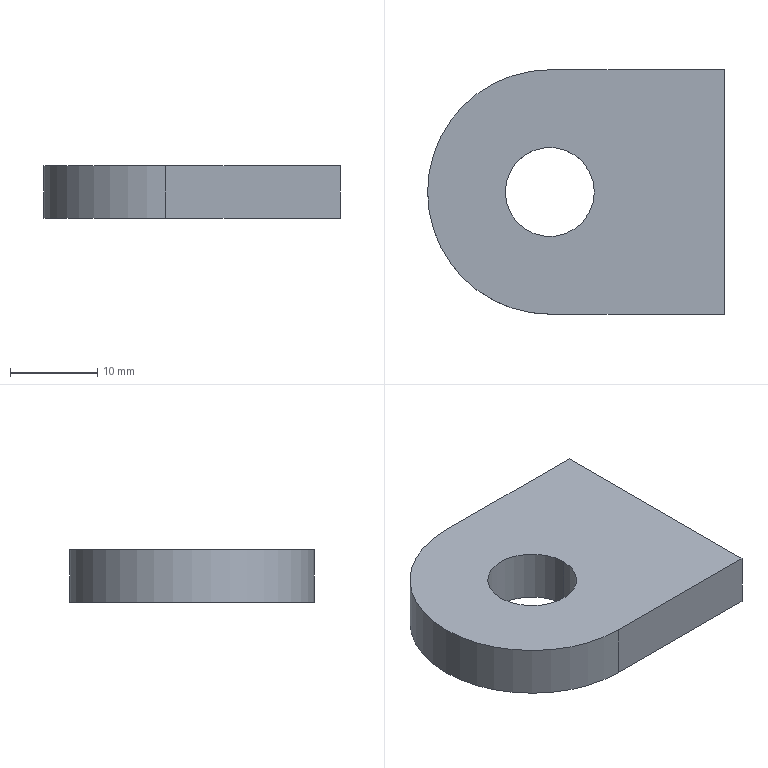Part | SolidWorks | features Extrusion 1 | 1 solid | 8 faces | box 34 x 28 x 6 mm | volume 4717 mm3 | plane 5 | cylinder 3 | commonest cylinder face diameters 10.2 x2 28 x1
STEP:
#1=CARTESIAN_POINT('',(-5.1,0.,-3.));
#2=VERTEX_POINT('',#1);
#3=CARTESIAN_POINT('',(5.1,0.,-3.));
#4=VERTEX_POINT('',#3);
#5=CARTESIAN_POINT('',(0.,0.,-3.));
#6=DIRECTION('',(0.,0.,1.));
#7=DIRECTION('',(1.,0.,0.));
#8=AXIS2_PLACEMENT_3D('',#5,#6,#7);
#9=CIRCLE('',#8,5.1);
#10=EDGE_CURVE('',#2,#4,#9,.T.);
#11=ORIENTED_EDGE('',*,*,#10,.F.);
#12=CARTESIAN_POINT('',(-5.1,0.,3.));
#13=VERTEX_POINT('',#12);
#14=CARTESIAN_POINT('',(-5.1,0.,-3.));
#15=DIRECTION('',(0.,0.,1.));
#16=VECTOR('',#15,1000.);
#17=LINE('',#14,#16);
#18=EDGE_CURVE('',#2,#13,#17,.T.);
#19=ORIENTED_EDGE('',*,*,#18,.T.);
#20=CARTESIAN_POINT('',(5.1,0.,3.));
#21=VERTEX_POINT('',#20);
#22=CARTESIAN_POINT('',(0.,0.,3.));
#23=DIRECTION('',(0.,0.,1.));
#24=DIRECTION('',(1.,0.,0.));
#25=AXIS2_PLACEMENT_3D('',#22,#23,#24);
#26=CIRCLE('',#25,5.1);
#27=EDGE_CURVE('',#13,#21,#26,.T.);
#28=ORIENTED_EDGE('',*,*,#27,.T.);
#29=CARTESIAN_POINT('',(5.1,0.,-3.));
#30=DIRECTION('',(0.,0.,1.));
#31=VECTOR('',#30,1000.);
#32=LINE('',#29,#31);
#33=EDGE_CURVE('',#4,#21,#32,.T.);
#34=ORIENTED_EDGE('',*,*,#33,.F.);
#35=EDGE_LOOP('',(#11,#19,#28,#34));
#36=FACE_OUTER_BOUND('',#35,.T.);
#37=CARTESIAN_POINT('',(0.,0.,-3.));
#38=DIRECTION('',(0.,0.,1.));
#39=DIRECTION('',(1.,0.,0.));
#40=AXIS2_PLACEMENT_3D('',#37,#38,#39);
#41=CYLINDRICAL_SURFACE('',#40,5.1);
#42=ADVANCED_FACE('',(#36),#41,.F.);
#43=CARTESIAN_POINT('',(0.,14.,3.));
#44=VERTEX_POINT('',#43);
#45=CARTESIAN_POINT('',(0.,-14.,3.));
#46=VERTEX_POINT('',#45);
#47=CARTESIAN_POINT('',(0.,0.,3.));
#48=DIRECTION('',(0.,0.,1.));
#49=DIRECTION('',(-1.,0.,0.));
#50=AXIS2_PLACEMENT_3D('',#47,#48,#49);
#51=CIRCLE('',#50,14.);
#52=EDGE_CURVE('',#44,#46,#51,.T.);
#53=ORIENTED_EDGE('',*,*,#52,.F.);
#54=CARTESIAN_POINT('',(0.,14.,-3.));
#55=VERTEX_POINT('',#54);
#56=CARTESIAN_POINT('',(0.,14.,-3.));
#57=DIRECTION('',(0.,0.,1.));
#58=VECTOR('',#57,1000.);
#59=LINE('',#56,#58);
#60=EDGE_CURVE('',#55,#44,#59,.T.);
#61=ORIENTED_EDGE('',*,*,#60,.F.);
#62=CARTESIAN_POINT('',(0.,-14.,-3.));
#63=VERTEX_POINT('',#62);
#64=CARTESIAN_POINT('',(0.,0.,-3.));
#65=DIRECTION('',(0.,0.,1.));
#66=DIRECTION('',(-1.,0.,0.));
#67=AXIS2_PLACEMENT_3D('',#64,#65,#66);
#68=CIRCLE('',#67,14.);
#69=EDGE_CURVE('',#55,#63,#68,.T.);
#70=ORIENTED_EDGE('',*,*,#69,.T.);
#71=CARTESIAN_POINT('',(0.,-14.,-3.));
#72=DIRECTION('',(0.,0.,1.));
#73=VECTOR('',#72,1000.);
#74=LINE('',#71,#73);
#75=EDGE_CURVE('',#63,#46,#74,.T.);
#76=ORIENTED_EDGE('',*,*,#75,.T.);
#77=EDGE_LOOP('',(#53,#61,#70,#76));
#78=FACE_OUTER_BOUND('',#77,.T.);
#79=CARTESIAN_POINT('',(0.,0.,-3.));
#80=DIRECTION('',(0.,0.,1.));
#81=DIRECTION('',(1.,0.,0.));
#82=AXIS2_PLACEMENT_3D('',#79,#80,#81);
#83=CYLINDRICAL_SURFACE('',#82,14.);
#84=ADVANCED_FACE('',(#78),#83,.T.);
#85=CARTESIAN_POINT('',(20.,14.,3.));
#86=VERTEX_POINT('',#85);
#87=CARTESIAN_POINT('',(0.,14.,3.));
#88=DIRECTION('',(-1.,0.,0.));
#89=VECTOR('',#88,1000.);
#90=LINE('',#87,#89);
#91=EDGE_CURVE('',#86,#44,#90,.T.);
#92=ORIENTED_EDGE('',*,*,#91,.F.);
#93=CARTESIAN_POINT('',(20.,14.,-3.));
#94=VERTEX_POINT('',#93);
#95=CARTESIAN_POINT('',(20.,14.,-3.));
#96=DIRECTION('',(0.,0.,1.));
#97=VECTOR('',#96,1000.);
#98=LINE('',#95,#97);
#99=EDGE_CURVE('',#94,#86,#98,.T.);
#100=ORIENTED_EDGE('',*,*,#99,.F.);
#101=CARTESIAN_POINT('',(0.,14.,-3.));
#102=DIRECTION('',(-1.,0.,0.));
#103=VECTOR('',#102,1000.);
#104=LINE('',#101,#103);
#105=EDGE_CURVE('',#94,#55,#104,.T.);
#106=ORIENTED_EDGE('',*,*,#105,.T.);
#107=ORIENTED_EDGE('',*,*,#60,.T.);
#108=EDGE_LOOP('',(#92,#100,#106,#107));
#109=FACE_OUTER_BOUND('',#108,.T.);
#110=CARTESIAN_POINT('',(0.,14.,-3.));
#111=DIRECTION('',(0.,1.,0.));
#112=DIRECTION('',(0.,0.,1.));
#113=AXIS2_PLACEMENT_3D('',#110,#111,#112);
#114=PLANE('',#113);
#115=ADVANCED_FACE('',(#109),#114,.T.);
#116=CARTESIAN_POINT('',(20.,-14.,3.));
#117=VERTEX_POINT('',#116);
#118=CARTESIAN_POINT('',(20.,14.,3.));
#119=DIRECTION('',(0.,1.,0.));
#120=VECTOR('',#119,1000.);
#121=LINE('',#118,#120);
#122=EDGE_CURVE('',#117,#86,#121,.T.);
#123=ORIENTED_EDGE('',*,*,#122,.F.);
#124=CARTESIAN_POINT('',(20.,-14.,-3.));
#125=VERTEX_POINT('',#124);
#126=CARTESIAN_POINT('',(20.,-14.,-3.));
#127=DIRECTION('',(0.,0.,1.));
#128=VECTOR('',#127,1000.);
#129=LINE('',#126,#128);
#130=EDGE_CURVE('',#125,#117,#129,.T.);
#131=ORIENTED_EDGE('',*,*,#130,.F.);
#132=CARTESIAN_POINT('',(20.,14.,-3.));
#133=DIRECTION('',(0.,1.,0.));
#134=VECTOR('',#133,1000.);
#135=LINE('',#132,#134);
#136=EDGE_CURVE('',#125,#94,#135,.T.);
#137=ORIENTED_EDGE('',*,*,#136,.T.);
#138=ORIENTED_EDGE('',*,*,#99,.T.);
#139=EDGE_LOOP('',(#123,#131,#137,#138));
#140=FACE_OUTER_BOUND('',#139,.T.);
#141=CARTESIAN_POINT('',(20.,14.,-3.));
#142=DIRECTION('',(1.,0.,0.));
#143=DIRECTION('',(0.,0.,-1.));
#144=AXIS2_PLACEMENT_3D('',#141,#142,#143);
#145=PLANE('',#144);
#146=ADVANCED_FACE('',(#140),#145,.T.);
#147=CARTESIAN_POINT('',(20.,-14.,3.));
#148=DIRECTION('',(1.,0.,0.));
#149=VECTOR('',#148,1000.);
#150=LINE('',#147,#149);
#151=EDGE_CURVE('',#46,#117,#150,.T.);
#152=ORIENTED_EDGE('',*,*,#151,.F.);
#153=ORIENTED_EDGE('',*,*,#75,.F.);
#154=CARTESIAN_POINT('',(20.,-14.,-3.));
#155=DIRECTION('',(1.,0.,0.));
#156=VECTOR('',#155,1000.);
#157=LINE('',#154,#156);
#158=EDGE_CURVE('',#63,#125,#157,.T.);
#159=ORIENTED_EDGE('',*,*,#158,.T.);
#160=ORIENTED_EDGE('',*,*,#130,.T.);
#161=EDGE_LOOP('',(#152,#153,#159,#160));
#162=FACE_OUTER_BOUND('',#161,.T.);
#163=CARTESIAN_POINT('',(20.,-14.,-3.));
#164=DIRECTION('',(0.,-1.,0.));
#165=DIRECTION('',(0.,0.,-1.));
#166=AXIS2_PLACEMENT_3D('',#163,#164,#165);
#167=PLANE('',#166);
#168=ADVANCED_FACE('',(#162),#167,.T.);
#169=CARTESIAN_POINT('',(0.,0.,-3.));
#170=DIRECTION('',(0.,0.,1.));
#171=DIRECTION('',(1.,0.,0.));
#172=AXIS2_PLACEMENT_3D('',#169,#170,#171);
#173=CIRCLE('',#172,5.1);
#174=EDGE_CURVE('',#4,#2,#173,.T.);
#175=ORIENTED_EDGE('',*,*,#174,.T.);
#176=ORIENTED_EDGE('',*,*,#10,.T.);
#177=EDGE_LOOP('',(#175,#176));
#178=FACE_BOUND('',#177,.T.);
#179=ORIENTED_EDGE('',*,*,#69,.F.);
#180=ORIENTED_EDGE('',*,*,#105,.F.);
#181=ORIENTED_EDGE('',*,*,#136,.F.);
#182=ORIENTED_EDGE('',*,*,#158,.F.);
#183=EDGE_LOOP('',(#179,#180,#181,#182));
#184=FACE_OUTER_BOUND('',#183,.T.);
#185=CARTESIAN_POINT('',(0.,0.,-3.));
#186=DIRECTION('',(0.,0.,-1.));
#187=DIRECTION('',(-1.,0.,0.));
#188=AXIS2_PLACEMENT_3D('',#185,#186,#187);
#189=PLANE('',#188);
#190=ADVANCED_FACE('',(#178,#184),#189,.T.);
#191=CARTESIAN_POINT('',(0.,0.,3.));
#192=DIRECTION('',(0.,0.,1.));
#193=DIRECTION('',(1.,0.,0.));
#194=AXIS2_PLACEMENT_3D('',#191,#192,#193);
#195=CIRCLE('',#194,5.1);
#196=EDGE_CURVE('',#21,#13,#195,.T.);
#197=ORIENTED_EDGE('',*,*,#196,.F.);
#198=ORIENTED_EDGE('',*,*,#27,.F.);
#199=EDGE_LOOP('',(#197,#198));
#200=FACE_BOUND('',#199,.T.);
#201=ORIENTED_EDGE('',*,*,#52,.T.);
#202=ORIENTED_EDGE('',*,*,#151,.T.);
#203=ORIENTED_EDGE('',*,*,#122,.T.);
#204=ORIENTED_EDGE('',*,*,#91,.T.);
#205=EDGE_LOOP('',(#201,#202,#203,#204));
#206=FACE_OUTER_BOUND('',#205,.T.);
#207=CARTESIAN_POINT('',(0.,0.,3.));
#208=DIRECTION('',(0.,0.,-1.));
#209=DIRECTION('',(-1.,0.,0.));
#210=AXIS2_PLACEMENT_3D('',#207,#208,#209);
#211=PLANE('',#210);
#212=ADVANCED_FACE('',(#200,#206),#211,.F.);
#213=ORIENTED_EDGE('',*,*,#18,.F.);
#214=ORIENTED_EDGE('',*,*,#174,.F.);
#215=ORIENTED_EDGE('',*,*,#33,.T.);
#216=ORIENTED_EDGE('',*,*,#196,.T.);
#217=EDGE_LOOP('',(#213,#214,#215,#216));
#218=FACE_OUTER_BOUND('',#217,.T.);
#219=CARTESIAN_POINT('',(0.,0.,-3.));
#220=DIRECTION('',(0.,0.,1.));
#221=DIRECTION('',(1.,0.,0.));
#222=AXIS2_PLACEMENT_3D('',#219,#220,#221);
#223=CYLINDRICAL_SURFACE('',#222,5.1);
#224=ADVANCED_FACE('',(#218),#223,.F.);
#225=CLOSED_SHELL('',(#42,#84,#115,#146,#168,#190,#212,#224));
#226=MANIFOLD_SOLID_BREP('',#225);
#227=CARTESIAN_POINT('',(0.,0.,0.));
#228=DIRECTION('',(0.,0.,1.));
#229=DIRECTION('',(1.,0.,0.));
#230=AXIS2_PLACEMENT_3D('',#227,#228,#229);
#231=(LENGTH_UNIT()NAMED_UNIT(*)SI_UNIT(.MILLI.,.METRE.));
#232=UNCERTAINTY_MEASURE_WITH_UNIT(LENGTH_MEASURE(0.00001),#231,'','');
#233=(NAMED_UNIT(*)PLANE_ANGLE_UNIT()SI_UNIT($,.RADIAN.));
#234=(NAMED_UNIT(*)SI_UNIT($,.STERADIAN.)SOLID_ANGLE_UNIT());
#235=(GEOMETRIC_REPRESENTATION_CONTEXT(3)GLOBAL_UNCERTAINTY_ASSIGNED_CONTEXT((#232))GLOBAL_UNIT_ASSIGNED_CONTEXT((#231,#233,#234))REPRESENTATION_CONTEXT('',''));
#236=ADVANCED_BREP_SHAPE_REPRESENTATION('',(#226,#230),#235);